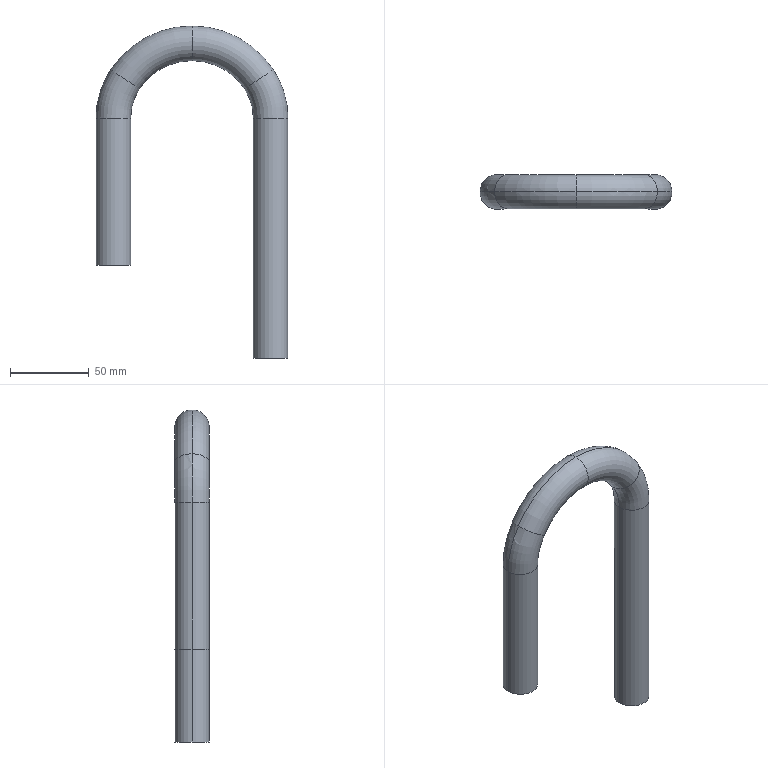Part | SolidWorks | features Sweep 1 | 1 solid | 26 faces | box 122 x 22 x 210.99 mm | volume 81123 mm3 | torus 16 | cylinder 8 | plane 2 | commonest cylinder face diameters 15 x4 22 x4
STEP:
#1=CARTESIAN_POINT('',(86.301,0.,113.95));
#2=VERTEX_POINT('',#1);
#3=CARTESIAN_POINT('',(98.822,0.,122.211));
#4=VERTEX_POINT('',#3);
#5=CARTESIAN_POINT('',(92.561,0.,118.081));
#6=DIRECTION('',(-0.5507,0.,0.8347));
#7=DIRECTION('',(-0.8347,0.,-0.5507));
#8=AXIS2_PLACEMENT_3D('',#5,#6,#7);
#9=CIRCLE('',#8,7.5);
#10=EDGE_CURVE('',#2,#4,#9,.T.);
#11=ORIENTED_EDGE('',*,*,#10,.T.);
#12=CARTESIAN_POINT('',(107.5,0.,93.299));
#13=VERTEX_POINT('',#12);
#14=CARTESIAN_POINT('',(55.,0.,93.299));
#15=DIRECTION('',(0.,1.,0.));
#16=DIRECTION('',(0.,0.,1.));
#17=AXIS2_PLACEMENT_3D('',#14,#15,#16);
#18=CIRCLE('',#17,52.5);
#19=EDGE_CURVE('',#4,#13,#18,.T.);
#20=ORIENTED_EDGE('',*,*,#19,.T.);
#21=CARTESIAN_POINT('',(92.5,0.,93.299));
#22=VERTEX_POINT('',#21);
#23=CARTESIAN_POINT('',(100.,0.,93.299));
#24=DIRECTION('',(0.,0.,1.));
#25=DIRECTION('',(-1.,0.,0.));
#26=AXIS2_PLACEMENT_3D('',#23,#24,#25);
#27=CIRCLE('',#26,7.5);
#28=EDGE_CURVE('',#22,#13,#27,.T.);
#29=ORIENTED_EDGE('',*,*,#28,.F.);
#30=CARTESIAN_POINT('',(55.,0.,93.299));
#31=DIRECTION('',(0.,1.,0.));
#32=DIRECTION('',(0.,0.,1.));
#33=AXIS2_PLACEMENT_3D('',#30,#31,#32);
#34=CIRCLE('',#33,37.5);
#35=EDGE_CURVE('',#2,#22,#34,.T.);
#36=ORIENTED_EDGE('',*,*,#35,.F.);
#37=EDGE_LOOP('',(#11,#20,#29,#36));
#38=FACE_OUTER_BOUND('',#37,.T.);
#39=CARTESIAN_POINT('',(55.,0.,93.299));
#40=DIRECTION('',(0.,1.,0.));
#41=DIRECTION('',(0.,0.,1.));
#42=AXIS2_PLACEMENT_3D('',#39,#40,#41);
#43=TOROIDAL_SURFACE('',#42,45.,7.5);
#44=ADVANCED_FACE('',(#38),#43,.F.);
#45=CARTESIAN_POINT('',(13.699,0.,113.95));
#46=VERTEX_POINT('',#45);
#47=CARTESIAN_POINT('',(1.178,0.,122.211));
#48=VERTEX_POINT('',#47);
#49=CARTESIAN_POINT('',(7.439,0.,118.081));
#50=DIRECTION('',(-0.5507,0.,-0.8347));
#51=DIRECTION('',(0.8347,0.,-0.5507));
#52=AXIS2_PLACEMENT_3D('',#49,#50,#51);
#53=CIRCLE('',#52,7.5);
#54=EDGE_CURVE('',#46,#48,#53,.T.);
#55=ORIENTED_EDGE('',*,*,#54,.T.);
#56=CARTESIAN_POINT('',(50.,0.,148.49));
#57=VERTEX_POINT('',#56);
#58=CARTESIAN_POINT('',(50.,0.,90.));
#59=DIRECTION('',(0.,1.,0.));
#60=DIRECTION('',(0.,0.,1.));
#61=AXIS2_PLACEMENT_3D('',#58,#59,#60);
#62=CIRCLE('',#61,58.49);
#63=EDGE_CURVE('',#48,#57,#62,.T.);
#64=ORIENTED_EDGE('',*,*,#63,.T.);
#65=CARTESIAN_POINT('',(50.,0.,133.49));
#66=VERTEX_POINT('',#65);
#67=CARTESIAN_POINT('',(50.,0.,140.99));
#68=DIRECTION('',(-1.,0.,0.));
#69=DIRECTION('',(0.,0.,1.));
#70=AXIS2_PLACEMENT_3D('',#67,#68,#69);
#71=CIRCLE('',#70,7.5);
#72=EDGE_CURVE('',#66,#57,#71,.T.);
#73=ORIENTED_EDGE('',*,*,#72,.F.);
#74=CARTESIAN_POINT('',(50.,0.,90.));
#75=DIRECTION('',(0.,1.,0.));
#76=DIRECTION('',(0.,0.,1.));
#77=AXIS2_PLACEMENT_3D('',#74,#75,#76);
#78=CIRCLE('',#77,43.49);
#79=EDGE_CURVE('',#46,#66,#78,.T.);
#80=ORIENTED_EDGE('',*,*,#79,.F.);
#81=EDGE_LOOP('',(#55,#64,#73,#80));
#82=FACE_OUTER_BOUND('',#81,.T.);
#83=CARTESIAN_POINT('',(50.,0.,90.));
#84=DIRECTION('',(0.,1.,0.));
#85=DIRECTION('',(0.,0.,1.));
#86=AXIS2_PLACEMENT_3D('',#83,#84,#85);
#87=TOROIDAL_SURFACE('',#86,50.99,7.5);
#88=ADVANCED_FACE('',(#82),#87,.F.);
#89=CARTESIAN_POINT('',(7.5,0.,93.299));
#90=VERTEX_POINT('',#89);
#91=CARTESIAN_POINT('',(-7.5,0.,93.299));
#92=VERTEX_POINT('',#91);
#93=CARTESIAN_POINT('',(0.,0.,93.299));
#94=DIRECTION('',(0.,0.,-1.));
#95=DIRECTION('',(1.,0.,0.));
#96=AXIS2_PLACEMENT_3D('',#93,#94,#95);
#97=CIRCLE('',#96,7.5);
#98=EDGE_CURVE('',#90,#92,#97,.T.);
#99=ORIENTED_EDGE('',*,*,#98,.T.);
#100=CARTESIAN_POINT('',(45.,0.,93.299));
#101=DIRECTION('',(0.,1.,0.));
#102=DIRECTION('',(0.,0.,1.));
#103=AXIS2_PLACEMENT_3D('',#100,#101,#102);
#104=CIRCLE('',#103,52.5);
#105=EDGE_CURVE('',#92,#48,#104,.T.);
#106=ORIENTED_EDGE('',*,*,#105,.T.);
#107=ORIENTED_EDGE('',*,*,#54,.F.);
#108=CARTESIAN_POINT('',(45.,0.,93.299));
#109=DIRECTION('',(0.,1.,0.));
#110=DIRECTION('',(0.,0.,1.));
#111=AXIS2_PLACEMENT_3D('',#108,#109,#110);
#112=CIRCLE('',#111,37.5);
#113=EDGE_CURVE('',#90,#46,#112,.T.);
#114=ORIENTED_EDGE('',*,*,#113,.F.);
#115=EDGE_LOOP('',(#99,#106,#107,#114));
#116=FACE_OUTER_BOUND('',#115,.T.);
#117=CARTESIAN_POINT('',(45.,0.,93.299));
#118=DIRECTION('',(0.,1.,0.));
#119=DIRECTION('',(0.,0.,1.));
#120=AXIS2_PLACEMENT_3D('',#117,#118,#119);
#121=TOROIDAL_SURFACE('',#120,45.,7.5);
#122=ADVANCED_FACE('',(#116),#121,.F.);
#123=CARTESIAN_POINT('',(83.38,0.,112.023));
#124=VERTEX_POINT('',#123);
#125=CARTESIAN_POINT('',(101.743,0.,124.139));
#126=VERTEX_POINT('',#125);
#127=CARTESIAN_POINT('',(92.561,0.,118.081));
#128=DIRECTION('',(0.5507,0.,-0.8347));
#129=DIRECTION('',(-0.8347,0.,-0.5507));
#130=AXIS2_PLACEMENT_3D('',#127,#128,#129);
#131=CIRCLE('',#130,11.);
#132=EDGE_CURVE('',#124,#126,#131,.T.);
#133=ORIENTED_EDGE('',*,*,#132,.T.);
#134=CARTESIAN_POINT('',(111.,0.,93.299));
#135=VERTEX_POINT('',#134);
#136=CARTESIAN_POINT('',(55.,0.,93.299));
#137=DIRECTION('',(0.,1.,0.));
#138=DIRECTION('',(0.,0.,1.));
#139=AXIS2_PLACEMENT_3D('',#136,#137,#138);
#140=CIRCLE('',#139,56.);
#141=EDGE_CURVE('',#126,#135,#140,.T.);
#142=ORIENTED_EDGE('',*,*,#141,.T.);
#143=CARTESIAN_POINT('',(89.,0.,93.299));
#144=VERTEX_POINT('',#143);
#145=CARTESIAN_POINT('',(100.,0.,93.299));
#146=DIRECTION('',(0.,0.,-1.));
#147=DIRECTION('',(-1.,0.,0.));
#148=AXIS2_PLACEMENT_3D('',#145,#146,#147);
#149=CIRCLE('',#148,11.);
#150=EDGE_CURVE('',#144,#135,#149,.T.);
#151=ORIENTED_EDGE('',*,*,#150,.F.);
#152=CARTESIAN_POINT('',(55.,0.,93.299));
#153=DIRECTION('',(0.,1.,0.));
#154=DIRECTION('',(0.,0.,1.));
#155=AXIS2_PLACEMENT_3D('',#152,#153,#154);
#156=CIRCLE('',#155,34.);
#157=EDGE_CURVE('',#124,#144,#156,.T.);
#158=ORIENTED_EDGE('',*,*,#157,.F.);
#159=EDGE_LOOP('',(#133,#142,#151,#158));
#160=FACE_OUTER_BOUND('',#159,.T.);
#161=CARTESIAN_POINT('',(55.,0.,93.299));
#162=DIRECTION('',(0.,1.,0.));
#163=DIRECTION('',(0.,0.,1.));
#164=AXIS2_PLACEMENT_3D('',#161,#162,#163);
#165=TOROIDAL_SURFACE('',#164,45.,11.);
#166=ADVANCED_FACE('',(#160),#165,.T.);
#167=CARTESIAN_POINT('',(50.,0.,151.99));
#168=VERTEX_POINT('',#167);
#169=CARTESIAN_POINT('',(50.,0.,129.99));
#170=VERTEX_POINT('',#169);
#171=CARTESIAN_POINT('',(50.,0.,140.99));
#172=DIRECTION('',(-1.,0.,0.));
#173=DIRECTION('',(0.,0.,1.));
#174=AXIS2_PLACEMENT_3D('',#171,#172,#173);
#175=CIRCLE('',#174,11.);
#176=EDGE_CURVE('',#168,#170,#175,.T.);
#177=ORIENTED_EDGE('',*,*,#176,.F.);
#178=CARTESIAN_POINT('',(50.,0.,90.));
#179=DIRECTION('',(0.,1.,0.));
#180=DIRECTION('',(0.,0.,1.));
#181=AXIS2_PLACEMENT_3D('',#178,#179,#180);
#182=CIRCLE('',#181,61.99);
#183=EDGE_CURVE('',#168,#126,#182,.T.);
#184=ORIENTED_EDGE('',*,*,#183,.T.);
#185=ORIENTED_EDGE('',*,*,#132,.F.);
#186=CARTESIAN_POINT('',(50.,0.,90.));
#187=DIRECTION('',(0.,1.,0.));
#188=DIRECTION('',(0.,0.,1.));
#189=AXIS2_PLACEMENT_3D('',#186,#187,#188);
#190=CIRCLE('',#189,39.99);
#191=EDGE_CURVE('',#170,#124,#190,.T.);
#192=ORIENTED_EDGE('',*,*,#191,.F.);
#193=EDGE_LOOP('',(#177,#184,#185,#192));
#194=FACE_OUTER_BOUND('',#193,.T.);
#195=CARTESIAN_POINT('',(50.,0.,90.));
#196=DIRECTION('',(0.,1.,0.));
#197=DIRECTION('',(0.,0.,1.));
#198=AXIS2_PLACEMENT_3D('',#195,#196,#197);
#199=TOROIDAL_SURFACE('',#198,50.99,11.);
#200=ADVANCED_FACE('',(#194),#199,.T.);
#201=CARTESIAN_POINT('',(11.,0.,93.299));
#202=VERTEX_POINT('',#201);
#203=CARTESIAN_POINT('',(-11.,0.,93.299));
#204=VERTEX_POINT('',#203);
#205=CARTESIAN_POINT('',(0.,0.,93.299));
#206=DIRECTION('',(0.,0.,1.));
#207=DIRECTION('',(1.,0.,0.));
#208=AXIS2_PLACEMENT_3D('',#205,#206,#207);
#209=CIRCLE('',#208,11.);
#210=EDGE_CURVE('',#202,#204,#209,.T.);
#211=ORIENTED_EDGE('',*,*,#210,.T.);
#212=CARTESIAN_POINT('',(-1.743,0.,124.139));
#213=VERTEX_POINT('',#212);
#214=CARTESIAN_POINT('',(45.,0.,93.299));
#215=DIRECTION('',(0.,1.,0.));
#216=DIRECTION('',(0.,0.,1.));
#217=AXIS2_PLACEMENT_3D('',#214,#215,#216);
#218=CIRCLE('',#217,56.);
#219=EDGE_CURVE('',#204,#213,#218,.T.);
#220=ORIENTED_EDGE('',*,*,#219,.T.);
#221=CARTESIAN_POINT('',(16.62,0.,112.023));
#222=VERTEX_POINT('',#221);
#223=CARTESIAN_POINT('',(7.439,0.,118.081));
#224=DIRECTION('',(0.5507,0.,0.8347));
#225=DIRECTION('',(0.8347,0.,-0.5507));
#226=AXIS2_PLACEMENT_3D('',#223,#224,#225);
#227=CIRCLE('',#226,11.);
#228=EDGE_CURVE('',#222,#213,#227,.T.);
#229=ORIENTED_EDGE('',*,*,#228,.F.);
#230=CARTESIAN_POINT('',(45.,0.,93.299));
#231=DIRECTION('',(0.,1.,0.));
#232=DIRECTION('',(0.,0.,1.));
#233=AXIS2_PLACEMENT_3D('',#230,#231,#232);
#234=CIRCLE('',#233,34.);
#235=EDGE_CURVE('',#202,#222,#234,.T.);
#236=ORIENTED_EDGE('',*,*,#235,.F.);
#237=EDGE_LOOP('',(#211,#220,#229,#236));
#238=FACE_OUTER_BOUND('',#237,.T.);
#239=CARTESIAN_POINT('',(45.,0.,93.299));
#240=DIRECTION('',(0.,1.,0.));
#241=DIRECTION('',(0.,0.,1.));
#242=AXIS2_PLACEMENT_3D('',#239,#240,#241);
#243=TOROIDAL_SURFACE('',#242,45.,11.);
#244=ADVANCED_FACE('',(#238),#243,.T.);
#245=ORIENTED_EDGE('',*,*,#228,.T.);
#246=CARTESIAN_POINT('',(50.,0.,90.));
#247=DIRECTION('',(0.,1.,0.));
#248=DIRECTION('',(0.,0.,1.));
#249=AXIS2_PLACEMENT_3D('',#246,#247,#248);
#250=CIRCLE('',#249,61.99);
#251=EDGE_CURVE('',#213,#168,#250,.T.);
#252=ORIENTED_EDGE('',*,*,#251,.T.);
#253=ORIENTED_EDGE('',*,*,#176,.T.);
#254=CARTESIAN_POINT('',(50.,0.,90.));
#255=DIRECTION('',(0.,1.,0.));
#256=DIRECTION('',(0.,0.,1.));
#257=AXIS2_PLACEMENT_3D('',#254,#255,#256);
#258=CIRCLE('',#257,39.99);
#259=EDGE_CURVE('',#222,#170,#258,.T.);
#260=ORIENTED_EDGE('',*,*,#259,.F.);
#261=EDGE_LOOP('',(#245,#252,#253,#260));
#262=FACE_OUTER_BOUND('',#261,.T.);
#263=CARTESIAN_POINT('',(50.,0.,90.));
#264=DIRECTION('',(0.,1.,0.));
#265=DIRECTION('',(0.,0.,1.));
#266=AXIS2_PLACEMENT_3D('',#263,#264,#265);
#267=TOROIDAL_SURFACE('',#266,50.99,11.);
#268=ADVANCED_FACE('',(#262),#267,.T.);
#269=ORIENTED_EDGE('',*,*,#72,.T.);
#270=CARTESIAN_POINT('',(50.,0.,90.));
#271=DIRECTION('',(0.,1.,0.));
#272=DIRECTION('',(0.,0.,1.));
#273=AXIS2_PLACEMENT_3D('',#270,#271,#272);
#274=CIRCLE('',#273,58.49);
#275=EDGE_CURVE('',#57,#4,#274,.T.);
#276=ORIENTED_EDGE('',*,*,#275,.T.);
#277=ORIENTED_EDGE('',*,*,#10,.F.);
#278=CARTESIAN_POINT('',(50.,0.,90.));
#279=DIRECTION('',(0.,1.,0.));
#280=DIRECTION('',(0.,0.,1.));
#281=AXIS2_PLACEMENT_3D('',#278,#279,#280);
#282=CIRCLE('',#281,43.49);
#283=EDGE_CURVE('',#66,#2,#282,.T.);
#284=ORIENTED_EDGE('',*,*,#283,.F.);
#285=EDGE_LOOP('',(#269,#276,#277,#284));
#286=FACE_OUTER_BOUND('',#285,.T.);
#287=CARTESIAN_POINT('',(50.,0.,90.));
#288=DIRECTION('',(0.,1.,0.));
#289=DIRECTION('',(0.,0.,1.));
#290=AXIS2_PLACEMENT_3D('',#287,#288,#289);
#291=TOROIDAL_SURFACE('',#290,50.99,7.5);
#292=ADVANCED_FACE('',(#286),#291,.F.);
#293=ORIENTED_EDGE('',*,*,#28,.T.);
#294=CARTESIAN_POINT('',(107.5,0.,-59.));
#295=VERTEX_POINT('',#294);
#296=CARTESIAN_POINT('',(107.5,0.,93.299));
#297=DIRECTION('',(0.,0.,-1.));
#298=VECTOR('',#297,1000.);
#299=LINE('',#296,#298);
#300=EDGE_CURVE('',#13,#295,#299,.T.);
#301=ORIENTED_EDGE('',*,*,#300,.T.);
#302=CARTESIAN_POINT('',(92.5,0.,-59.));
#303=VERTEX_POINT('',#302);
#304=CARTESIAN_POINT('',(100.,0.,-59.));
#305=DIRECTION('',(0.,0.,1.));
#306=DIRECTION('',(-1.,0.,0.));
#307=AXIS2_PLACEMENT_3D('',#304,#305,#306);
#308=CIRCLE('',#307,7.5);
#309=EDGE_CURVE('',#303,#295,#308,.T.);
#310=ORIENTED_EDGE('',*,*,#309,.F.);
#311=CARTESIAN_POINT('',(92.5,0.,93.299));
#312=DIRECTION('',(0.,0.,-1.));
#313=VECTOR('',#312,1000.);
#314=LINE('',#311,#313);
#315=EDGE_CURVE('',#22,#303,#314,.T.);
#316=ORIENTED_EDGE('',*,*,#315,.F.);
#317=EDGE_LOOP('',(#293,#301,#310,#316));
#318=FACE_OUTER_BOUND('',#317,.T.);
#319=CARTESIAN_POINT('',(100.,0.,93.299));
#320=DIRECTION('',(0.,0.,-1.));
#321=DIRECTION('',(-1.,0.,0.));
#322=AXIS2_PLACEMENT_3D('',#319,#320,#321);
#323=CYLINDRICAL_SURFACE('',#322,7.5);
#324=ADVANCED_FACE('',(#318),#323,.F.);
#325=ORIENTED_EDGE('',*,*,#275,.F.);
#326=CARTESIAN_POINT('',(50.,0.,140.99));
#327=DIRECTION('',(-1.,0.,0.));
#328=DIRECTION('',(0.,0.,1.));
#329=AXIS2_PLACEMENT_3D('',#326,#327,#328);
#330=CIRCLE('',#329,7.5);
#331=EDGE_CURVE('',#57,#66,#330,.T.);
#332=ORIENTED_EDGE('',*,*,#331,.T.);
#333=ORIENTED_EDGE('',*,*,#283,.T.);
#334=CARTESIAN_POINT('',(92.561,0.,118.081));
#335=DIRECTION('',(-0.5507,0.,0.8347));
#336=DIRECTION('',(-0.8347,0.,-0.5507));
#337=AXIS2_PLACEMENT_3D('',#334,#335,#336);
#338=CIRCLE('',#337,7.5);
#339=EDGE_CURVE('',#4,#2,#338,.T.);
#340=ORIENTED_EDGE('',*,*,#339,.F.);
#341=EDGE_LOOP('',(#325,#332,#333,#340));
#342=FACE_OUTER_BOUND('',#341,.T.);
#343=CARTESIAN_POINT('',(50.,0.,90.));
#344=DIRECTION('',(0.,1.,0.));
#345=DIRECTION('',(0.,0.,1.));
#346=AXIS2_PLACEMENT_3D('',#343,#344,#345);
#347=TOROIDAL_SURFACE('',#346,50.99,7.5);
#348=ADVANCED_FACE('',(#342),#347,.F.);
#349=CARTESIAN_POINT('',(7.5,0.,0.));
#350=VERTEX_POINT('',#349);
#351=CARTESIAN_POINT('',(-7.5,0.,0.));
#352=VERTEX_POINT('',#351);
#353=CARTESIAN_POINT('',(0.,0.,0.));
#354=DIRECTION('',(0.,0.,-1.));
#355=DIRECTION('',(1.,0.,0.));
#356=AXIS2_PLACEMENT_3D('',#353,#354,#355);
#357=CIRCLE('',#356,7.5);
#358=EDGE_CURVE('',#350,#352,#357,.T.);
#359=ORIENTED_EDGE('',*,*,#358,.T.);
#360=CARTESIAN_POINT('',(-7.5,0.,0.));
#361=DIRECTION('',(0.,0.,1.));
#362=VECTOR('',#361,1000.);
#363=LINE('',#360,#362);
#364=EDGE_CURVE('',#352,#92,#363,.T.);
#365=ORIENTED_EDGE('',*,*,#364,.T.);
#366=ORIENTED_EDGE('',*,*,#98,.F.);
#367=CARTESIAN_POINT('',(7.5,0.,0.));
#368=DIRECTION('',(0.,0.,1.));
#369=VECTOR('',#368,1000.);
#370=LINE('',#367,#369);
#371=EDGE_CURVE('',#350,#90,#370,.T.);
#372=ORIENTED_EDGE('',*,*,#371,.F.);
#373=EDGE_LOOP('',(#359,#365,#366,#372));
#374=FACE_OUTER_BOUND('',#373,.T.);
#375=CARTESIAN_POINT('',(0.,0.,0.));
#376=DIRECTION('',(0.,0.,1.));
#377=DIRECTION('',(1.,0.,0.));
#378=AXIS2_PLACEMENT_3D('',#375,#376,#377);
#379=CYLINDRICAL_SURFACE('',#378,7.5);
#380=ADVANCED_FACE('',(#374),#379,.F.);
#381=ORIENTED_EDGE('',*,*,#150,.T.);
#382=CARTESIAN_POINT('',(111.,0.,-59.));
#383=VERTEX_POINT('',#382);
#384=CARTESIAN_POINT('',(111.,0.,93.299));
#385=DIRECTION('',(0.,0.,-1.));
#386=VECTOR('',#385,1000.);
#387=LINE('',#384,#386);
#388=EDGE_CURVE('',#135,#383,#387,.T.);
#389=ORIENTED_EDGE('',*,*,#388,.T.);
#390=CARTESIAN_POINT('',(89.,0.,-59.));
#391=VERTEX_POINT('',#390);
#392=CARTESIAN_POINT('',(100.,0.,-59.));
#393=DIRECTION('',(0.,0.,-1.));
#394=DIRECTION('',(-1.,0.,0.));
#395=AXIS2_PLACEMENT_3D('',#392,#393,#394);
#396=CIRCLE('',#395,11.);
#397=EDGE_CURVE('',#391,#383,#396,.T.);
#398=ORIENTED_EDGE('',*,*,#397,.F.);
#399=CARTESIAN_POINT('',(89.,0.,93.299));
#400=DIRECTION('',(0.,0.,-1.));
#401=VECTOR('',#400,1000.);
#402=LINE('',#399,#401);
#403=EDGE_CURVE('',#144,#391,#402,.T.);
#404=ORIENTED_EDGE('',*,*,#403,.F.);
#405=EDGE_LOOP('',(#381,#389,#398,#404));
#406=FACE_OUTER_BOUND('',#405,.T.);
#407=CARTESIAN_POINT('',(100.,0.,93.299));
#408=DIRECTION('',(0.,0.,-1.));
#409=DIRECTION('',(-1.,0.,0.));
#410=AXIS2_PLACEMENT_3D('',#407,#408,#409);
#411=CYLINDRICAL_SURFACE('',#410,11.);
#412=ADVANCED_FACE('',(#406),#411,.T.);
#413=ORIENTED_EDGE('',*,*,#251,.F.);
#414=CARTESIAN_POINT('',(7.439,0.,118.081));
#415=DIRECTION('',(0.5507,0.,0.8347));
#416=DIRECTION('',(0.8347,0.,-0.5507));
#417=AXIS2_PLACEMENT_3D('',#414,#415,#416);
#418=CIRCLE('',#417,11.);
#419=EDGE_CURVE('',#213,#222,#418,.T.);
#420=ORIENTED_EDGE('',*,*,#419,.T.);
#421=ORIENTED_EDGE('',*,*,#259,.T.);
#422=CARTESIAN_POINT('',(50.,0.,140.99));
#423=DIRECTION('',(-1.,0.,0.));
#424=DIRECTION('',(0.,0.,1.));
#425=AXIS2_PLACEMENT_3D('',#422,#423,#424);
#426=CIRCLE('',#425,11.);
#427=EDGE_CURVE('',#170,#168,#426,.T.);
#428=ORIENTED_EDGE('',*,*,#427,.T.);
#429=EDGE_LOOP('',(#413,#420,#421,#428));
#430=FACE_OUTER_BOUND('',#429,.T.);
#431=CARTESIAN_POINT('',(50.,0.,90.));
#432=DIRECTION('',(0.,1.,0.));
#433=DIRECTION('',(0.,0.,1.));
#434=AXIS2_PLACEMENT_3D('',#431,#432,#433);
#435=TOROIDAL_SURFACE('',#434,50.99,11.);
#436=ADVANCED_FACE('',(#430),#435,.T.);
#437=CARTESIAN_POINT('',(11.,0.,0.));
#438=VERTEX_POINT('',#437);
#439=CARTESIAN_POINT('',(-11.,0.,0.));
#440=VERTEX_POINT('',#439);
#441=CARTESIAN_POINT('',(0.,0.,0.));
#442=DIRECTION('',(0.,0.,1.));
#443=DIRECTION('',(1.,0.,0.));
#444=AXIS2_PLACEMENT_3D('',#441,#442,#443);
#445=CIRCLE('',#444,11.);
#446=EDGE_CURVE('',#438,#440,#445,.T.);
#447=ORIENTED_EDGE('',*,*,#446,.T.);
#448=CARTESIAN_POINT('',(-11.,0.,0.));
#449=DIRECTION('',(0.,0.,1.));
#450=VECTOR('',#449,1000.);
#451=LINE('',#448,#450);
#452=EDGE_CURVE('',#440,#204,#451,.T.);
#453=ORIENTED_EDGE('',*,*,#452,.T.);
#454=ORIENTED_EDGE('',*,*,#210,.F.);
#455=CARTESIAN_POINT('',(11.,0.,0.));
#456=DIRECTION('',(0.,0.,1.));
#457=VECTOR('',#456,1000.);
#458=LINE('',#455,#457);
#459=EDGE_CURVE('',#438,#202,#458,.T.);
#460=ORIENTED_EDGE('',*,*,#459,.F.);
#461=EDGE_LOOP('',(#447,#453,#454,#460));
#462=FACE_OUTER_BOUND('',#461,.T.);
#463=CARTESIAN_POINT('',(0.,0.,0.));
#464=DIRECTION('',(0.,0.,1.));
#465=DIRECTION('',(1.,0.,0.));
#466=AXIS2_PLACEMENT_3D('',#463,#464,#465);
#467=CYLINDRICAL_SURFACE('',#466,11.);
#468=ADVANCED_FACE('',(#462),#467,.T.);
#469=ORIENTED_EDGE('',*,*,#300,.F.);
#470=CARTESIAN_POINT('',(100.,0.,93.299));
#471=DIRECTION('',(0.,0.,1.));
#472=DIRECTION('',(-1.,0.,0.));
#473=AXIS2_PLACEMENT_3D('',#470,#471,#472);
#474=CIRCLE('',#473,7.5);
#475=EDGE_CURVE('',#13,#22,#474,.T.);
#476=ORIENTED_EDGE('',*,*,#475,.T.);
#477=ORIENTED_EDGE('',*,*,#315,.T.);
#478=CARTESIAN_POINT('',(100.,0.,-59.));
#479=DIRECTION('',(0.,0.,1.));
#480=DIRECTION('',(-1.,0.,0.));
#481=AXIS2_PLACEMENT_3D('',#478,#479,#480);
#482=CIRCLE('',#481,7.5);
#483=EDGE_CURVE('',#295,#303,#482,.T.);
#484=ORIENTED_EDGE('',*,*,#483,.F.);
#485=EDGE_LOOP('',(#469,#476,#477,#484));
#486=FACE_OUTER_BOUND('',#485,.T.);
#487=CARTESIAN_POINT('',(100.,0.,93.299));
#488=DIRECTION('',(0.,0.,-1.));
#489=DIRECTION('',(-1.,0.,0.));
#490=AXIS2_PLACEMENT_3D('',#487,#488,#489);
#491=CYLINDRICAL_SURFACE('',#490,7.5);
#492=ADVANCED_FACE('',(#486),#491,.F.);
#493=ORIENTED_EDGE('',*,*,#19,.F.);
#494=ORIENTED_EDGE('',*,*,#339,.T.);
#495=ORIENTED_EDGE('',*,*,#35,.T.);
#496=ORIENTED_EDGE('',*,*,#475,.F.);
#497=EDGE_LOOP('',(#493,#494,#495,#496));
#498=FACE_OUTER_BOUND('',#497,.T.);
#499=CARTESIAN_POINT('',(55.,0.,93.299));
#500=DIRECTION('',(0.,1.,0.));
#501=DIRECTION('',(0.,0.,1.));
#502=AXIS2_PLACEMENT_3D('',#499,#500,#501);
#503=TOROIDAL_SURFACE('',#502,45.,7.5);
#504=ADVANCED_FACE('',(#498),#503,.F.);
#505=ORIENTED_EDGE('',*,*,#63,.F.);
#506=CARTESIAN_POINT('',(7.439,0.,118.081));
#507=DIRECTION('',(-0.5507,0.,-0.8347));
#508=DIRECTION('',(0.8347,0.,-0.5507));
#509=AXIS2_PLACEMENT_3D('',#506,#507,#508);
#510=CIRCLE('',#509,7.5);
#511=EDGE_CURVE('',#48,#46,#510,.T.);
#512=ORIENTED_EDGE('',*,*,#511,.T.);
#513=ORIENTED_EDGE('',*,*,#79,.T.);
#514=ORIENTED_EDGE('',*,*,#331,.F.);
#515=EDGE_LOOP('',(#505,#512,#513,#514));
#516=FACE_OUTER_BOUND('',#515,.T.);
#517=CARTESIAN_POINT('',(50.,0.,90.));
#518=DIRECTION('',(0.,1.,0.));
#519=DIRECTION('',(0.,0.,1.));
#520=AXIS2_PLACEMENT_3D('',#517,#518,#519);
#521=TOROIDAL_SURFACE('',#520,50.99,7.5);
#522=ADVANCED_FACE('',(#516),#521,.F.);
#523=ORIENTED_EDGE('',*,*,#105,.F.);
#524=CARTESIAN_POINT('',(0.,0.,93.299));
#525=DIRECTION('',(0.,0.,-1.));
#526=DIRECTION('',(1.,0.,0.));
#527=AXIS2_PLACEMENT_3D('',#524,#525,#526);
#528=CIRCLE('',#527,7.5);
#529=EDGE_CURVE('',#92,#90,#528,.T.);
#530=ORIENTED_EDGE('',*,*,#529,.T.);
#531=ORIENTED_EDGE('',*,*,#113,.T.);
#532=ORIENTED_EDGE('',*,*,#511,.F.);
#533=EDGE_LOOP('',(#523,#530,#531,#532));
#534=FACE_OUTER_BOUND('',#533,.T.);
#535=CARTESIAN_POINT('',(45.,0.,93.299));
#536=DIRECTION('',(0.,1.,0.));
#537=DIRECTION('',(0.,0.,1.));
#538=AXIS2_PLACEMENT_3D('',#535,#536,#537);
#539=TOROIDAL_SURFACE('',#538,45.,7.5);
#540=ADVANCED_FACE('',(#534),#539,.F.);
#541=ORIENTED_EDGE('',*,*,#364,.F.);
#542=CARTESIAN_POINT('',(0.,0.,0.));
#543=DIRECTION('',(0.,0.,-1.));
#544=DIRECTION('',(1.,0.,0.));
#545=AXIS2_PLACEMENT_3D('',#542,#543,#544);
#546=CIRCLE('',#545,7.5);
#547=EDGE_CURVE('',#352,#350,#546,.T.);
#548=ORIENTED_EDGE('',*,*,#547,.T.);
#549=ORIENTED_EDGE('',*,*,#371,.T.);
#550=ORIENTED_EDGE('',*,*,#529,.F.);
#551=EDGE_LOOP('',(#541,#548,#549,#550));
#552=FACE_OUTER_BOUND('',#551,.T.);
#553=CARTESIAN_POINT('',(0.,0.,0.));
#554=DIRECTION('',(0.,0.,1.));
#555=DIRECTION('',(1.,0.,0.));
#556=AXIS2_PLACEMENT_3D('',#553,#554,#555);
#557=CYLINDRICAL_SURFACE('',#556,7.5);
#558=ADVANCED_FACE('',(#552),#557,.F.);
#559=ORIENTED_EDGE('',*,*,#309,.T.);
#560=ORIENTED_EDGE('',*,*,#483,.T.);
#561=EDGE_LOOP('',(#559,#560));
#562=FACE_BOUND('',#561,.T.);
#563=ORIENTED_EDGE('',*,*,#397,.T.);
#564=CARTESIAN_POINT('',(100.,0.,-59.));
#565=DIRECTION('',(0.,0.,-1.));
#566=DIRECTION('',(-1.,0.,0.));
#567=AXIS2_PLACEMENT_3D('',#564,#565,#566);
#568=CIRCLE('',#567,11.);
#569=EDGE_CURVE('',#383,#391,#568,.T.);
#570=ORIENTED_EDGE('',*,*,#569,.T.);
#571=EDGE_LOOP('',(#563,#570));
#572=FACE_OUTER_BOUND('',#571,.T.);
#573=CARTESIAN_POINT('',(100.,0.,-59.));
#574=DIRECTION('',(0.,0.,-1.));
#575=DIRECTION('',(-1.,0.,0.));
#576=AXIS2_PLACEMENT_3D('',#573,#574,#575);
#577=PLANE('',#576);
#578=ADVANCED_FACE('',(#562,#572),#577,.T.);
#579=ORIENTED_EDGE('',*,*,#358,.F.);
#580=ORIENTED_EDGE('',*,*,#547,.F.);
#581=EDGE_LOOP('',(#579,#580));
#582=FACE_BOUND('',#581,.T.);
#583=ORIENTED_EDGE('',*,*,#446,.F.);
#584=CARTESIAN_POINT('',(0.,0.,0.));
#585=DIRECTION('',(0.,0.,1.));
#586=DIRECTION('',(1.,0.,0.));
#587=AXIS2_PLACEMENT_3D('',#584,#585,#586);
#588=CIRCLE('',#587,11.);
#589=EDGE_CURVE('',#440,#438,#588,.T.);
#590=ORIENTED_EDGE('',*,*,#589,.F.);
#591=EDGE_LOOP('',(#583,#590));
#592=FACE_OUTER_BOUND('',#591,.T.);
#593=CARTESIAN_POINT('',(0.,0.,0.));
#594=DIRECTION('',(0.,0.,1.));
#595=DIRECTION('',(1.,0.,0.));
#596=AXIS2_PLACEMENT_3D('',#593,#594,#595);
#597=PLANE('',#596);
#598=ADVANCED_FACE('',(#582,#592),#597,.F.);
#599=ORIENTED_EDGE('',*,*,#388,.F.);
#600=CARTESIAN_POINT('',(100.,0.,93.299));
#601=DIRECTION('',(0.,0.,-1.));
#602=DIRECTION('',(-1.,0.,0.));
#603=AXIS2_PLACEMENT_3D('',#600,#601,#602);
#604=CIRCLE('',#603,11.);
#605=EDGE_CURVE('',#135,#144,#604,.T.);
#606=ORIENTED_EDGE('',*,*,#605,.T.);
#607=ORIENTED_EDGE('',*,*,#403,.T.);
#608=ORIENTED_EDGE('',*,*,#569,.F.);
#609=EDGE_LOOP('',(#599,#606,#607,#608));
#610=FACE_OUTER_BOUND('',#609,.T.);
#611=CARTESIAN_POINT('',(100.,0.,93.299));
#612=DIRECTION('',(0.,0.,-1.));
#613=DIRECTION('',(-1.,0.,0.));
#614=AXIS2_PLACEMENT_3D('',#611,#612,#613);
#615=CYLINDRICAL_SURFACE('',#614,11.);
#616=ADVANCED_FACE('',(#610),#615,.T.);
#617=ORIENTED_EDGE('',*,*,#141,.F.);
#618=CARTESIAN_POINT('',(92.561,0.,118.081));
#619=DIRECTION('',(0.5507,0.,-0.8347));
#620=DIRECTION('',(-0.8347,0.,-0.5507));
#621=AXIS2_PLACEMENT_3D('',#618,#619,#620);
#622=CIRCLE('',#621,11.);
#623=EDGE_CURVE('',#126,#124,#622,.T.);
#624=ORIENTED_EDGE('',*,*,#623,.T.);
#625=ORIENTED_EDGE('',*,*,#157,.T.);
#626=ORIENTED_EDGE('',*,*,#605,.F.);
#627=EDGE_LOOP('',(#617,#624,#625,#626));
#628=FACE_OUTER_BOUND('',#627,.T.);
#629=CARTESIAN_POINT('',(55.,0.,93.299));
#630=DIRECTION('',(0.,1.,0.));
#631=DIRECTION('',(0.,0.,1.));
#632=AXIS2_PLACEMENT_3D('',#629,#630,#631);
#633=TOROIDAL_SURFACE('',#632,45.,11.);
#634=ADVANCED_FACE('',(#628),#633,.T.);
#635=ORIENTED_EDGE('',*,*,#183,.F.);
#636=ORIENTED_EDGE('',*,*,#427,.F.);
#637=ORIENTED_EDGE('',*,*,#191,.T.);
#638=ORIENTED_EDGE('',*,*,#623,.F.);
#639=EDGE_LOOP('',(#635,#636,#637,#638));
#640=FACE_OUTER_BOUND('',#639,.T.);
#641=CARTESIAN_POINT('',(50.,0.,90.));
#642=DIRECTION('',(0.,1.,0.));
#643=DIRECTION('',(0.,0.,1.));
#644=AXIS2_PLACEMENT_3D('',#641,#642,#643);
#645=TOROIDAL_SURFACE('',#644,50.99,11.);
#646=ADVANCED_FACE('',(#640),#645,.T.);
#647=ORIENTED_EDGE('',*,*,#219,.F.);
#648=CARTESIAN_POINT('',(0.,0.,93.299));
#649=DIRECTION('',(0.,0.,1.));
#650=DIRECTION('',(1.,0.,0.));
#651=AXIS2_PLACEMENT_3D('',#648,#649,#650);
#652=CIRCLE('',#651,11.);
#653=EDGE_CURVE('',#204,#202,#652,.T.);
#654=ORIENTED_EDGE('',*,*,#653,.T.);
#655=ORIENTED_EDGE('',*,*,#235,.T.);
#656=ORIENTED_EDGE('',*,*,#419,.F.);
#657=EDGE_LOOP('',(#647,#654,#655,#656));
#658=FACE_OUTER_BOUND('',#657,.T.);
#659=CARTESIAN_POINT('',(45.,0.,93.299));
#660=DIRECTION('',(0.,1.,0.));
#661=DIRECTION('',(0.,0.,1.));
#662=AXIS2_PLACEMENT_3D('',#659,#660,#661);
#663=TOROIDAL_SURFACE('',#662,45.,11.);
#664=ADVANCED_FACE('',(#658),#663,.T.);
#665=ORIENTED_EDGE('',*,*,#452,.F.);
#666=ORIENTED_EDGE('',*,*,#589,.T.);
#667=ORIENTED_EDGE('',*,*,#459,.T.);
#668=ORIENTED_EDGE('',*,*,#653,.F.);
#669=EDGE_LOOP('',(#665,#666,#667,#668));
#670=FACE_OUTER_BOUND('',#669,.T.);
#671=CARTESIAN_POINT('',(0.,0.,0.));
#672=DIRECTION('',(0.,0.,1.));
#673=DIRECTION('',(1.,0.,0.));
#674=AXIS2_PLACEMENT_3D('',#671,#672,#673);
#675=CYLINDRICAL_SURFACE('',#674,11.);
#676=ADVANCED_FACE('',(#670),#675,.T.);
#677=CLOSED_SHELL('',(#44,#88,#122,#166,#200,#244,#268,#292,#324,#348,#380,#412,#436,#468,#492,#504,#522,#540,#558,#578,#598,#616,#634,#646,#664,#676));
#678=MANIFOLD_SOLID_BREP('',#677);
#679=CARTESIAN_POINT('',(0.,0.,0.));
#680=DIRECTION('',(0.,0.,1.));
#681=DIRECTION('',(1.,0.,0.));
#682=AXIS2_PLACEMENT_3D('',#679,#680,#681);
#683=(LENGTH_UNIT()NAMED_UNIT(*)SI_UNIT(.MILLI.,.METRE.));
#684=UNCERTAINTY_MEASURE_WITH_UNIT(LENGTH_MEASURE(0.00001),#683,'','');
#685=(NAMED_UNIT(*)PLANE_ANGLE_UNIT()SI_UNIT($,.RADIAN.));
#686=(NAMED_UNIT(*)SI_UNIT($,.STERADIAN.)SOLID_ANGLE_UNIT());
#687=(GEOMETRIC_REPRESENTATION_CONTEXT(3)GLOBAL_UNCERTAINTY_ASSIGNED_CONTEXT((#684))GLOBAL_UNIT_ASSIGNED_CONTEXT((#683,#685,#686))REPRESENTATION_CONTEXT('',''));
#688=ADVANCED_BREP_SHAPE_REPRESENTATION('',(#678,#682),#687);